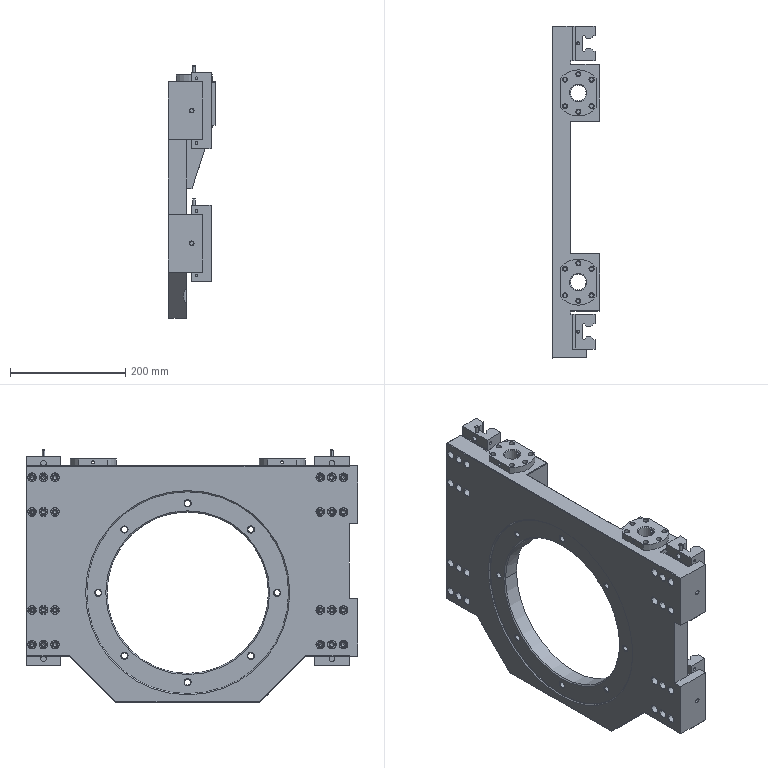Part | SolidWorks | 7 solids | 895 faces | box 82 x 575 x 437.9 mm | volume 6520185 mm3 | cone 323 | cylinder 304 | plane 266 | spline 2 | commonest cylinder face diameters 5 x48 6.8 x48 8.5 x48 14 x48 6.5 x28 9 x24